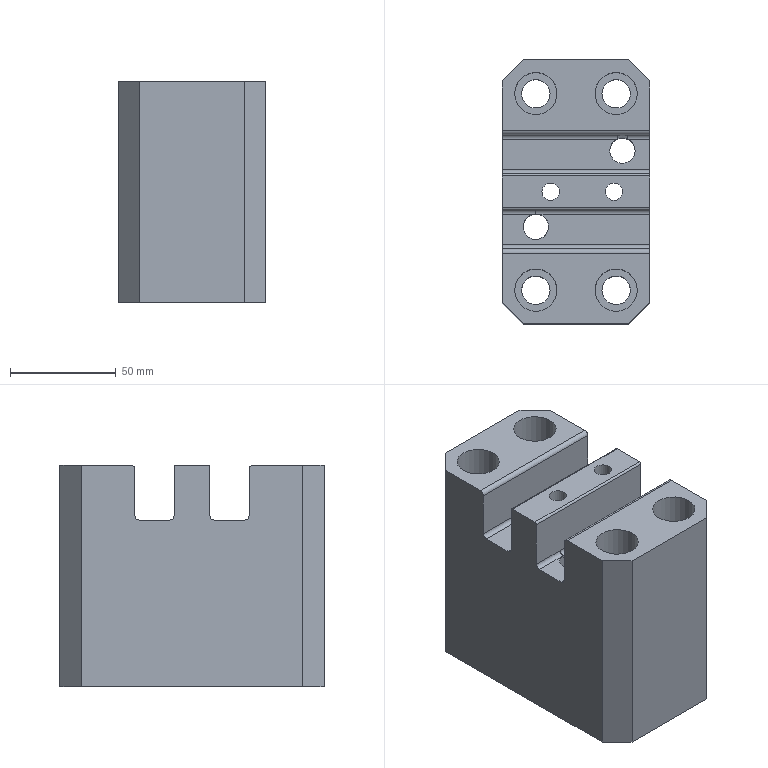Part | STEP file | lll_id4830_x_t | 1 solid | 54 faces | box 70 x 125 x 105 mm | volume 687764 mm3 | plane 28 | cylinder 24 | spline 2 | commonest cylinder face diameters 4 x8 13.509 x4 20.008 x4 2 x2 8.2 x2 12 x2